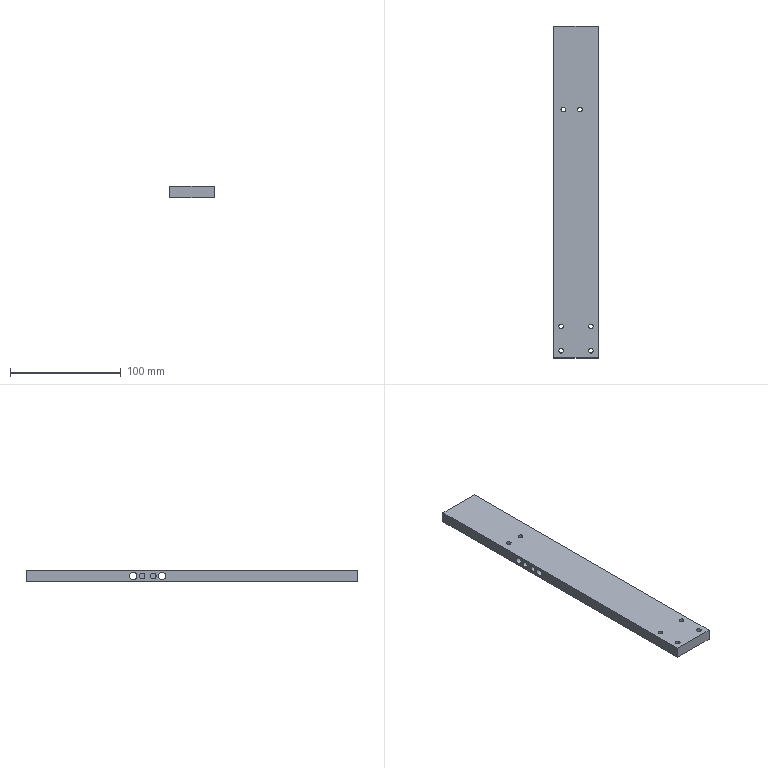Part | STEP file | 11-FG-B04811 | 1 solid | 36 faces | box 40 x 300 x 10 mm | volume 115513 mm3 | cylinder 24 | plane 8 | cone 4 | commonest cylinder face diameters 4.2 x12 5 x8 6.5 x4
STEP:
#1=CARTESIAN_POINT('',(-9.4,224.5,5.));
#2=VERTEX_POINT('',#1);
#3=CARTESIAN_POINT('',(-13.6,224.5,5.));
#4=VERTEX_POINT('',#3);
#5=CARTESIAN_POINT('',(-11.5,224.5,5.));
#6=DIRECTION('',(0.,0.,-1.));
#7=DIRECTION('',(-1.,0.,0.));
#8=AXIS2_PLACEMENT_3D('',#5,#6,#7);
#9=CIRCLE('',#8,2.1);
#10=EDGE_CURVE('',#2,#4,#9,.T.);
#11=ORIENTED_EDGE('',*,*,#10,.F.);
#12=CARTESIAN_POINT('',(-9.4,224.5,-5.));
#13=VERTEX_POINT('',#12);
#14=CARTESIAN_POINT('',(-9.4,224.5,-5.));
#15=DIRECTION('',(0.,0.,-1.));
#16=VECTOR('',#15,1000.);
#17=LINE('',#14,#16);
#18=EDGE_CURVE('',#2,#13,#17,.T.);
#19=ORIENTED_EDGE('',*,*,#18,.T.);
#20=CARTESIAN_POINT('',(-13.6,224.5,-5.));
#21=VERTEX_POINT('',#20);
#22=CARTESIAN_POINT('',(-11.5,224.5,-5.));
#23=DIRECTION('',(0.,0.,-1.));
#24=DIRECTION('',(-1.,0.,0.));
#25=AXIS2_PLACEMENT_3D('',#22,#23,#24);
#26=CIRCLE('',#25,2.1);
#27=EDGE_CURVE('',#13,#21,#26,.T.);
#28=ORIENTED_EDGE('',*,*,#27,.T.);
#29=CARTESIAN_POINT('',(-13.6,224.5,-5.));
#30=DIRECTION('',(0.,0.,-1.));
#31=VECTOR('',#30,1000.);
#32=LINE('',#29,#31);
#33=EDGE_CURVE('',#4,#21,#32,.T.);
#34=ORIENTED_EDGE('',*,*,#33,.F.);
#35=EDGE_LOOP('',(#11,#19,#28,#34));
#36=FACE_OUTER_BOUND('',#35,.T.);
#37=CARTESIAN_POINT('',(-11.5,224.5,-5.));
#38=DIRECTION('',(0.,0.,-1.));
#39=DIRECTION('',(-1.,0.,0.));
#40=AXIS2_PLACEMENT_3D('',#37,#38,#39);
#41=CYLINDRICAL_SURFACE('',#40,2.1);
#42=ADVANCED_FACE('',(#36),#41,.F.);
#43=CARTESIAN_POINT('',(5.6,224.5,5.));
#44=VERTEX_POINT('',#43);
#45=CARTESIAN_POINT('',(1.4,224.5,5.));
#46=VERTEX_POINT('',#45);
#47=CARTESIAN_POINT('',(3.5,224.5,5.));
#48=DIRECTION('',(0.,0.,-1.));
#49=DIRECTION('',(-1.,0.,0.));
#50=AXIS2_PLACEMENT_3D('',#47,#48,#49);
#51=CIRCLE('',#50,2.1);
#52=EDGE_CURVE('',#44,#46,#51,.T.);
#53=ORIENTED_EDGE('',*,*,#52,.F.);
#54=CARTESIAN_POINT('',(5.6,224.5,-5.));
#55=VERTEX_POINT('',#54);
#56=CARTESIAN_POINT('',(5.6,224.5,-5.));
#57=DIRECTION('',(0.,0.,-1.));
#58=VECTOR('',#57,1000.);
#59=LINE('',#56,#58);
#60=EDGE_CURVE('',#44,#55,#59,.T.);
#61=ORIENTED_EDGE('',*,*,#60,.T.);
#62=CARTESIAN_POINT('',(1.4,224.5,-5.));
#63=VERTEX_POINT('',#62);
#64=CARTESIAN_POINT('',(3.5,224.5,-5.));
#65=DIRECTION('',(0.,0.,-1.));
#66=DIRECTION('',(-1.,0.,0.));
#67=AXIS2_PLACEMENT_3D('',#64,#65,#66);
#68=CIRCLE('',#67,2.1);
#69=EDGE_CURVE('',#55,#63,#68,.T.);
#70=ORIENTED_EDGE('',*,*,#69,.T.);
#71=CARTESIAN_POINT('',(1.4,224.5,-5.));
#72=DIRECTION('',(0.,0.,-1.));
#73=VECTOR('',#72,1000.);
#74=LINE('',#71,#73);
#75=EDGE_CURVE('',#46,#63,#74,.T.);
#76=ORIENTED_EDGE('',*,*,#75,.F.);
#77=EDGE_LOOP('',(#53,#61,#70,#76));
#78=FACE_OUTER_BOUND('',#77,.T.);
#79=CARTESIAN_POINT('',(3.5,224.5,-5.));
#80=DIRECTION('',(0.,0.,-1.));
#81=DIRECTION('',(-1.,0.,0.));
#82=AXIS2_PLACEMENT_3D('',#79,#80,#81);
#83=CYLINDRICAL_SURFACE('',#82,2.1);
#84=ADVANCED_FACE('',(#78),#83,.F.);
#85=CARTESIAN_POINT('',(11.4,6.5,-5.));
#86=VERTEX_POINT('',#85);
#87=CARTESIAN_POINT('',(15.6,6.5,-5.));
#88=VERTEX_POINT('',#87);
#89=CARTESIAN_POINT('',(13.5,6.5,-5.));
#90=DIRECTION('',(0.,0.,1.));
#91=DIRECTION('',(1.,0.,0.));
#92=AXIS2_PLACEMENT_3D('',#89,#90,#91);
#93=CIRCLE('',#92,2.1);
#94=EDGE_CURVE('',#86,#88,#93,.T.);
#95=ORIENTED_EDGE('',*,*,#94,.F.);
#96=CARTESIAN_POINT('',(11.4,6.5,5.));
#97=VERTEX_POINT('',#96);
#98=CARTESIAN_POINT('',(11.4,6.5,5.));
#99=DIRECTION('',(0.,0.,1.));
#100=VECTOR('',#99,1000.);
#101=LINE('',#98,#100);
#102=EDGE_CURVE('',#86,#97,#101,.T.);
#103=ORIENTED_EDGE('',*,*,#102,.T.);
#104=CARTESIAN_POINT('',(15.6,6.5,5.));
#105=VERTEX_POINT('',#104);
#106=CARTESIAN_POINT('',(13.5,6.5,5.));
#107=DIRECTION('',(0.,0.,1.));
#108=DIRECTION('',(1.,0.,0.));
#109=AXIS2_PLACEMENT_3D('',#106,#107,#108);
#110=CIRCLE('',#109,2.1);
#111=EDGE_CURVE('',#97,#105,#110,.T.);
#112=ORIENTED_EDGE('',*,*,#111,.T.);
#113=CARTESIAN_POINT('',(15.6,6.5,5.));
#114=DIRECTION('',(0.,0.,1.));
#115=VECTOR('',#114,1000.);
#116=LINE('',#113,#115);
#117=EDGE_CURVE('',#88,#105,#116,.T.);
#118=ORIENTED_EDGE('',*,*,#117,.F.);
#119=EDGE_LOOP('',(#95,#103,#112,#118));
#120=FACE_OUTER_BOUND('',#119,.T.);
#121=CARTESIAN_POINT('',(13.5,6.5,5.));
#122=DIRECTION('',(0.,0.,1.));
#123=DIRECTION('',(1.,0.,0.));
#124=AXIS2_PLACEMENT_3D('',#121,#122,#123);
#125=CYLINDRICAL_SURFACE('',#124,2.1);
#126=ADVANCED_FACE('',(#120),#125,.F.);
#127=CARTESIAN_POINT('',(11.4,28.5,-5.));
#128=VERTEX_POINT('',#127);
#129=CARTESIAN_POINT('',(15.6,28.5,-5.));
#130=VERTEX_POINT('',#129);
#131=CARTESIAN_POINT('',(13.5,28.5,-5.));
#132=DIRECTION('',(0.,0.,1.));
#133=DIRECTION('',(1.,0.,0.));
#134=AXIS2_PLACEMENT_3D('',#131,#132,#133);
#135=CIRCLE('',#134,2.1);
#136=EDGE_CURVE('',#128,#130,#135,.T.);
#137=ORIENTED_EDGE('',*,*,#136,.F.);
#138=CARTESIAN_POINT('',(11.4,28.5,5.));
#139=VERTEX_POINT('',#138);
#140=CARTESIAN_POINT('',(11.4,28.5,5.));
#141=DIRECTION('',(0.,0.,1.));
#142=VECTOR('',#141,1000.);
#143=LINE('',#140,#142);
#144=EDGE_CURVE('',#128,#139,#143,.T.);
#145=ORIENTED_EDGE('',*,*,#144,.T.);
#146=CARTESIAN_POINT('',(15.6,28.5,5.));
#147=VERTEX_POINT('',#146);
#148=CARTESIAN_POINT('',(13.5,28.5,5.));
#149=DIRECTION('',(0.,0.,1.));
#150=DIRECTION('',(1.,0.,0.));
#151=AXIS2_PLACEMENT_3D('',#148,#149,#150);
#152=CIRCLE('',#151,2.1);
#153=EDGE_CURVE('',#139,#147,#152,.T.);
#154=ORIENTED_EDGE('',*,*,#153,.T.);
#155=CARTESIAN_POINT('',(15.6,28.5,5.));
#156=DIRECTION('',(0.,0.,1.));
#157=VECTOR('',#156,1000.);
#158=LINE('',#155,#157);
#159=EDGE_CURVE('',#130,#147,#158,.T.);
#160=ORIENTED_EDGE('',*,*,#159,.F.);
#161=EDGE_LOOP('',(#137,#145,#154,#160));
#162=FACE_OUTER_BOUND('',#161,.T.);
#163=CARTESIAN_POINT('',(13.5,28.5,5.));
#164=DIRECTION('',(0.,0.,1.));
#165=DIRECTION('',(1.,0.,0.));
#166=AXIS2_PLACEMENT_3D('',#163,#164,#165);
#167=CYLINDRICAL_SURFACE('',#166,2.1);
#168=ADVANCED_FACE('',(#162),#167,.F.);
#169=CARTESIAN_POINT('',(-15.6,28.5,-5.));
#170=VERTEX_POINT('',#169);
#171=CARTESIAN_POINT('',(-11.4,28.5,-5.));
#172=VERTEX_POINT('',#171);
#173=CARTESIAN_POINT('',(-13.5,28.5,-5.));
#174=DIRECTION('',(0.,0.,1.));
#175=DIRECTION('',(1.,0.,0.));
#176=AXIS2_PLACEMENT_3D('',#173,#174,#175);
#177=CIRCLE('',#176,2.1);
#178=EDGE_CURVE('',#170,#172,#177,.T.);
#179=ORIENTED_EDGE('',*,*,#178,.F.);
#180=CARTESIAN_POINT('',(-15.6,28.5,5.));
#181=VERTEX_POINT('',#180);
#182=CARTESIAN_POINT('',(-15.6,28.5,5.));
#183=DIRECTION('',(0.,0.,1.));
#184=VECTOR('',#183,1000.);
#185=LINE('',#182,#184);
#186=EDGE_CURVE('',#170,#181,#185,.T.);
#187=ORIENTED_EDGE('',*,*,#186,.T.);
#188=CARTESIAN_POINT('',(-11.4,28.5,5.));
#189=VERTEX_POINT('',#188);
#190=CARTESIAN_POINT('',(-13.5,28.5,5.));
#191=DIRECTION('',(0.,0.,1.));
#192=DIRECTION('',(1.,0.,0.));
#193=AXIS2_PLACEMENT_3D('',#190,#191,#192);
#194=CIRCLE('',#193,2.1);
#195=EDGE_CURVE('',#181,#189,#194,.T.);
#196=ORIENTED_EDGE('',*,*,#195,.T.);
#197=CARTESIAN_POINT('',(-11.4,28.5,5.));
#198=DIRECTION('',(0.,0.,1.));
#199=VECTOR('',#198,1000.);
#200=LINE('',#197,#199);
#201=EDGE_CURVE('',#172,#189,#200,.T.);
#202=ORIENTED_EDGE('',*,*,#201,.F.);
#203=EDGE_LOOP('',(#179,#187,#196,#202));
#204=FACE_OUTER_BOUND('',#203,.T.);
#205=CARTESIAN_POINT('',(-13.5,28.5,5.));
#206=DIRECTION('',(0.,0.,1.));
#207=DIRECTION('',(1.,0.,0.));
#208=AXIS2_PLACEMENT_3D('',#205,#206,#207);
#209=CYLINDRICAL_SURFACE('',#208,2.1);
#210=ADVANCED_FACE('',(#204),#209,.F.);
#211=CARTESIAN_POINT('',(-15.6,6.5,-5.));
#212=VERTEX_POINT('',#211);
#213=CARTESIAN_POINT('',(-11.4,6.5,-5.));
#214=VERTEX_POINT('',#213);
#215=CARTESIAN_POINT('',(-13.5,6.5,-5.));
#216=DIRECTION('',(0.,0.,1.));
#217=DIRECTION('',(1.,0.,0.));
#218=AXIS2_PLACEMENT_3D('',#215,#216,#217);
#219=CIRCLE('',#218,2.1);
#220=EDGE_CURVE('',#212,#214,#219,.T.);
#221=ORIENTED_EDGE('',*,*,#220,.F.);
#222=CARTESIAN_POINT('',(-15.6,6.5,5.));
#223=VERTEX_POINT('',#222);
#224=CARTESIAN_POINT('',(-15.6,6.5,5.));
#225=DIRECTION('',(0.,0.,1.));
#226=VECTOR('',#225,1000.);
#227=LINE('',#224,#226);
#228=EDGE_CURVE('',#212,#223,#227,.T.);
#229=ORIENTED_EDGE('',*,*,#228,.T.);
#230=CARTESIAN_POINT('',(-11.4,6.5,5.));
#231=VERTEX_POINT('',#230);
#232=CARTESIAN_POINT('',(-13.5,6.5,5.));
#233=DIRECTION('',(0.,0.,1.));
#234=DIRECTION('',(1.,0.,0.));
#235=AXIS2_PLACEMENT_3D('',#232,#233,#234);
#236=CIRCLE('',#235,2.1);
#237=EDGE_CURVE('',#223,#231,#236,.T.);
#238=ORIENTED_EDGE('',*,*,#237,.T.);
#239=CARTESIAN_POINT('',(-11.4,6.5,5.));
#240=DIRECTION('',(0.,0.,1.));
#241=VECTOR('',#240,1000.);
#242=LINE('',#239,#241);
#243=EDGE_CURVE('',#214,#231,#242,.T.);
#244=ORIENTED_EDGE('',*,*,#243,.F.);
#245=EDGE_LOOP('',(#221,#229,#238,#244));
#246=FACE_OUTER_BOUND('',#245,.T.);
#247=CARTESIAN_POINT('',(-13.5,6.5,5.));
#248=DIRECTION('',(0.,0.,1.));
#249=DIRECTION('',(1.,0.,0.));
#250=AXIS2_PLACEMENT_3D('',#247,#248,#249);
#251=CYLINDRICAL_SURFACE('',#250,2.1);
#252=ADVANCED_FACE('',(#246),#251,.F.);
#253=CARTESIAN_POINT('',(-12.,285.,-2.5));
#254=VERTEX_POINT('',#253);
#255=CARTESIAN_POINT('',(-12.,285.,2.5));
#256=VERTEX_POINT('',#255);
#257=CARTESIAN_POINT('',(-12.,285.,0.));
#258=DIRECTION('',(0.,1.,0.));
#259=DIRECTION('',(0.,0.,1.));
#260=AXIS2_PLACEMENT_3D('',#257,#258,#259);
#261=CIRCLE('',#260,2.5);
#262=EDGE_CURVE('',#254,#256,#261,.T.);
#263=ORIENTED_EDGE('',*,*,#262,.F.);
#264=CARTESIAN_POINT('',(-12.,300.,-2.5));
#265=VERTEX_POINT('',#264);
#266=CARTESIAN_POINT('',(-12.,300.,-2.5));
#267=DIRECTION('',(0.,1.,0.));
#268=VECTOR('',#267,1000.);
#269=LINE('',#266,#268);
#270=EDGE_CURVE('',#254,#265,#269,.T.);
#271=ORIENTED_EDGE('',*,*,#270,.T.);
#272=CARTESIAN_POINT('',(-12.,300.,2.5));
#273=VERTEX_POINT('',#272);
#274=CARTESIAN_POINT('',(-12.,300.,0.));
#275=DIRECTION('',(0.,1.,0.));
#276=DIRECTION('',(0.,0.,1.));
#277=AXIS2_PLACEMENT_3D('',#274,#275,#276);
#278=CIRCLE('',#277,2.5);
#279=EDGE_CURVE('',#265,#273,#278,.T.);
#280=ORIENTED_EDGE('',*,*,#279,.T.);
#281=CARTESIAN_POINT('',(-12.,300.,2.5));
#282=DIRECTION('',(0.,1.,0.));
#283=VECTOR('',#282,1000.);
#284=LINE('',#281,#283);
#285=EDGE_CURVE('',#256,#273,#284,.T.);
#286=ORIENTED_EDGE('',*,*,#285,.F.);
#287=EDGE_LOOP('',(#263,#271,#280,#286));
#288=FACE_OUTER_BOUND('',#287,.T.);
#289=CARTESIAN_POINT('',(-12.,300.,0.));
#290=DIRECTION('',(0.,1.,0.));
#291=DIRECTION('',(0.,0.,1.));
#292=AXIS2_PLACEMENT_3D('',#289,#290,#291);
#293=CYLINDRICAL_SURFACE('',#292,2.5);
#294=ADVANCED_FACE('',(#288),#293,.F.);
#295=CARTESIAN_POINT('',(-12.,283.498,0.));
#296=VERTEX_POINT('',#295);
#297=CARTESIAN_POINT('',(-12.,285.,2.5));
#298=DIRECTION('',(0.,0.515,0.8572));
#299=VECTOR('',#298,1000.);
#300=LINE('',#297,#299);
#301=EDGE_CURVE('',#296,#256,#300,.T.);
#302=ORIENTED_EDGE('',*,*,#301,.F.);
#303=CARTESIAN_POINT('',(-12.,285.,-2.5));
#304=DIRECTION('',(0.,0.515,-0.8572));
#305=VECTOR('',#304,1000.);
#306=LINE('',#303,#305);
#307=EDGE_CURVE('',#296,#254,#306,.T.);
#308=ORIENTED_EDGE('',*,*,#307,.T.);
#309=ORIENTED_EDGE('',*,*,#262,.T.);
#310=EDGE_LOOP('',(#302,#308,#309));
#311=FACE_OUTER_BOUND('',#310,.T.);
#312=CARTESIAN_POINT('',(-12.,285.,0.));
#313=DIRECTION('',(0.,1.,0.));
#314=DIRECTION('',(0.,0.,1.));
#315=AXIS2_PLACEMENT_3D('',#312,#313,#314);
#316=CONICAL_SURFACE('',#315,2.5,1.03);
#317=ADVANCED_FACE('',(#311),#316,.F.);
#318=CARTESIAN_POINT('',(12.,285.,-2.5));
#319=VERTEX_POINT('',#318);
#320=CARTESIAN_POINT('',(12.,285.,2.5));
#321=VERTEX_POINT('',#320);
#322=CARTESIAN_POINT('',(12.,285.,0.));
#323=DIRECTION('',(0.,1.,0.));
#324=DIRECTION('',(0.,0.,1.));
#325=AXIS2_PLACEMENT_3D('',#322,#323,#324);
#326=CIRCLE('',#325,2.5);
#327=EDGE_CURVE('',#319,#321,#326,.T.);
#328=ORIENTED_EDGE('',*,*,#327,.F.);
#329=CARTESIAN_POINT('',(12.,300.,-2.5));
#330=VERTEX_POINT('',#329);
#331=CARTESIAN_POINT('',(12.,300.,-2.5));
#332=DIRECTION('',(0.,1.,0.));
#333=VECTOR('',#332,1000.);
#334=LINE('',#331,#333);
#335=EDGE_CURVE('',#319,#330,#334,.T.);
#336=ORIENTED_EDGE('',*,*,#335,.T.);
#337=CARTESIAN_POINT('',(12.,300.,2.5));
#338=VERTEX_POINT('',#337);
#339=CARTESIAN_POINT('',(12.,300.,0.));
#340=DIRECTION('',(0.,1.,0.));
#341=DIRECTION('',(0.,0.,1.));
#342=AXIS2_PLACEMENT_3D('',#339,#340,#341);
#343=CIRCLE('',#342,2.5);
#344=EDGE_CURVE('',#330,#338,#343,.T.);
#345=ORIENTED_EDGE('',*,*,#344,.T.);
#346=CARTESIAN_POINT('',(12.,300.,2.5));
#347=DIRECTION('',(0.,1.,0.));
#348=VECTOR('',#347,1000.);
#349=LINE('',#346,#348);
#350=EDGE_CURVE('',#321,#338,#349,.T.);
#351=ORIENTED_EDGE('',*,*,#350,.F.);
#352=EDGE_LOOP('',(#328,#336,#345,#351));
#353=FACE_OUTER_BOUND('',#352,.T.);
#354=CARTESIAN_POINT('',(12.,300.,0.));
#355=DIRECTION('',(0.,1.,0.));
#356=DIRECTION('',(0.,0.,1.));
#357=AXIS2_PLACEMENT_3D('',#354,#355,#356);
#358=CYLINDRICAL_SURFACE('',#357,2.5);
#359=ADVANCED_FACE('',(#353),#358,.F.);
#360=CARTESIAN_POINT('',(12.,283.498,0.));
#361=VERTEX_POINT('',#360);
#362=CARTESIAN_POINT('',(12.,285.,2.5));
#363=DIRECTION('',(0.,0.515,0.8572));
#364=VECTOR('',#363,1000.);
#365=LINE('',#362,#364);
#366=EDGE_CURVE('',#361,#321,#365,.T.);
#367=ORIENTED_EDGE('',*,*,#366,.F.);
#368=CARTESIAN_POINT('',(12.,285.,-2.5));
#369=DIRECTION('',(0.,0.515,-0.8572));
#370=VECTOR('',#369,1000.);
#371=LINE('',#368,#370);
#372=EDGE_CURVE('',#361,#319,#371,.T.);
#373=ORIENTED_EDGE('',*,*,#372,.T.);
#374=ORIENTED_EDGE('',*,*,#327,.T.);
#375=EDGE_LOOP('',(#367,#373,#374));
#376=FACE_OUTER_BOUND('',#375,.T.);
#377=CARTESIAN_POINT('',(12.,285.,0.));
#378=DIRECTION('',(0.,1.,0.));
#379=DIRECTION('',(0.,0.,1.));
#380=AXIS2_PLACEMENT_3D('',#377,#378,#379);
#381=CONICAL_SURFACE('',#380,2.5,1.03);
#382=ADVANCED_FACE('',(#376),#381,.F.);
#383=CARTESIAN_POINT('',(-10.,195.,-2.5));
#384=VERTEX_POINT('',#383);
#385=CARTESIAN_POINT('',(-10.,195.,2.5));
#386=VERTEX_POINT('',#385);
#387=CARTESIAN_POINT('',(-10.,195.,0.));
#388=DIRECTION('',(-1.,0.,0.));
#389=DIRECTION('',(0.,0.,1.));
#390=AXIS2_PLACEMENT_3D('',#387,#388,#389);
#391=CIRCLE('',#390,2.5);
#392=EDGE_CURVE('',#384,#386,#391,.T.);
#393=ORIENTED_EDGE('',*,*,#392,.F.);
#394=CARTESIAN_POINT('',(-20.,195.,-2.5));
#395=VERTEX_POINT('',#394);
#396=CARTESIAN_POINT('',(-10.,195.,-2.5));
#397=DIRECTION('',(-1.,0.,0.));
#398=VECTOR('',#397,1000.);
#399=LINE('',#396,#398);
#400=EDGE_CURVE('',#384,#395,#399,.T.);
#401=ORIENTED_EDGE('',*,*,#400,.T.);
#402=CARTESIAN_POINT('',(-20.,195.,2.5));
#403=VERTEX_POINT('',#402);
#404=CARTESIAN_POINT('',(-20.,195.,0.));
#405=DIRECTION('',(-1.,0.,0.));
#406=DIRECTION('',(0.,0.,1.));
#407=AXIS2_PLACEMENT_3D('',#404,#405,#406);
#408=CIRCLE('',#407,2.5);
#409=EDGE_CURVE('',#395,#403,#408,.T.);
#410=ORIENTED_EDGE('',*,*,#409,.T.);
#411=CARTESIAN_POINT('',(-10.,195.,2.5));
#412=DIRECTION('',(-1.,0.,0.));
#413=VECTOR('',#412,1000.);
#414=LINE('',#411,#413);
#415=EDGE_CURVE('',#386,#403,#414,.T.);
#416=ORIENTED_EDGE('',*,*,#415,.F.);
#417=EDGE_LOOP('',(#393,#401,#410,#416));
#418=FACE_OUTER_BOUND('',#417,.T.);
#419=CARTESIAN_POINT('',(-10.,195.,0.));
#420=DIRECTION('',(-1.,0.,0.));
#421=DIRECTION('',(0.,0.,1.));
#422=AXIS2_PLACEMENT_3D('',#419,#420,#421);
#423=CYLINDRICAL_SURFACE('',#422,2.5);
#424=ADVANCED_FACE('',(#418),#423,.F.);
#425=CARTESIAN_POINT('',(-10.,185.,-2.5));
#426=VERTEX_POINT('',#425);
#427=CARTESIAN_POINT('',(-10.,185.,2.5));
#428=VERTEX_POINT('',#427);
#429=CARTESIAN_POINT('',(-10.,185.,0.));
#430=DIRECTION('',(-1.,0.,0.));
#431=DIRECTION('',(0.,0.,1.));
#432=AXIS2_PLACEMENT_3D('',#429,#430,#431);
#433=CIRCLE('',#432,2.5);
#434=EDGE_CURVE('',#426,#428,#433,.T.);
#435=ORIENTED_EDGE('',*,*,#434,.F.);
#436=CARTESIAN_POINT('',(-20.,185.,-2.5));
#437=VERTEX_POINT('',#436);
#438=CARTESIAN_POINT('',(-10.,185.,-2.5));
#439=DIRECTION('',(-1.,0.,0.));
#440=VECTOR('',#439,1000.);
#441=LINE('',#438,#440);
#442=EDGE_CURVE('',#426,#437,#441,.T.);
#443=ORIENTED_EDGE('',*,*,#442,.T.);
#444=CARTESIAN_POINT('',(-20.,185.,2.5));
#445=VERTEX_POINT('',#444);
#446=CARTESIAN_POINT('',(-20.,185.,0.));
#447=DIRECTION('',(-1.,0.,0.));
#448=DIRECTION('',(0.,0.,1.));
#449=AXIS2_PLACEMENT_3D('',#446,#447,#448);
#450=CIRCLE('',#449,2.5);
#451=EDGE_CURVE('',#437,#445,#450,.T.);
#452=ORIENTED_EDGE('',*,*,#451,.T.);
#453=CARTESIAN_POINT('',(-10.,185.,2.5));
#454=DIRECTION('',(-1.,0.,0.));
#455=VECTOR('',#454,1000.);
#456=LINE('',#453,#455);
#457=EDGE_CURVE('',#428,#445,#456,.T.);
#458=ORIENTED_EDGE('',*,*,#457,.F.);
#459=EDGE_LOOP('',(#435,#443,#452,#458));
#460=FACE_OUTER_BOUND('',#459,.T.);
#461=CARTESIAN_POINT('',(-10.,185.,0.));
#462=DIRECTION('',(-1.,0.,0.));
#463=DIRECTION('',(0.,0.,1.));
#464=AXIS2_PLACEMENT_3D('',#461,#462,#463);
#465=CYLINDRICAL_SURFACE('',#464,2.5);
#466=ADVANCED_FACE('',(#460),#465,.F.);
#467=CARTESIAN_POINT('',(-20.,177.,3.25));
#468=VERTEX_POINT('',#467);
#469=CARTESIAN_POINT('',(-20.,177.,-3.25));
#470=VERTEX_POINT('',#469);
#471=CARTESIAN_POINT('',(-20.,177.,0.));
#472=DIRECTION('',(1.,0.,0.));
#473=DIRECTION('',(0.,0.,-1.));
#474=AXIS2_PLACEMENT_3D('',#471,#472,#473);
#475=CIRCLE('',#474,3.25);
#476=EDGE_CURVE('',#468,#470,#475,.T.);
#477=ORIENTED_EDGE('',*,*,#476,.F.);
#478=CARTESIAN_POINT('',(20.,177.,3.25));
#479=VERTEX_POINT('',#478);
#480=CARTESIAN_POINT('',(-85.,177.,3.25));
#481=DIRECTION('',(1.,0.,0.));
#482=VECTOR('',#481,1000.);
#483=LINE('',#480,#482);
#484=EDGE_CURVE('',#468,#479,#483,.T.);
#485=ORIENTED_EDGE('',*,*,#484,.T.);
#486=CARTESIAN_POINT('',(20.,177.,-3.25));
#487=VERTEX_POINT('',#486);
#488=CARTESIAN_POINT('',(20.,177.,0.));
#489=DIRECTION('',(1.,0.,0.));
#490=DIRECTION('',(0.,0.,-1.));
#491=AXIS2_PLACEMENT_3D('',#488,#489,#490);
#492=CIRCLE('',#491,3.25);
#493=EDGE_CURVE('',#479,#487,#492,.T.);
#494=ORIENTED_EDGE('',*,*,#493,.T.);
#495=CARTESIAN_POINT('',(-85.,177.,-3.25));
#496=DIRECTION('',(1.,0.,0.));
#497=VECTOR('',#496,1000.);
#498=LINE('',#495,#497);
#499=EDGE_CURVE('',#470,#487,#498,.T.);
#500=ORIENTED_EDGE('',*,*,#499,.F.);
#501=EDGE_LOOP('',(#477,#485,#494,#500));
#502=FACE_OUTER_BOUND('',#501,.T.);
#503=CARTESIAN_POINT('',(-85.,177.,0.));
#504=DIRECTION('',(1.,0.,0.));
#505=DIRECTION('',(0.,0.,-1.));
#506=AXIS2_PLACEMENT_3D('',#503,#504,#505);
#507=CYLINDRICAL_SURFACE('',#506,3.25);
#508=ADVANCED_FACE('',(#502),#507,.F.);
#509=CARTESIAN_POINT('',(-20.,203.,3.25));
#510=VERTEX_POINT('',#509);
#511=CARTESIAN_POINT('',(-20.,203.,-3.25));
#512=VERTEX_POINT('',#511);
#513=CARTESIAN_POINT('',(-20.,203.,0.));
#514=DIRECTION('',(1.,0.,0.));
#515=DIRECTION('',(0.,0.,-1.));
#516=AXIS2_PLACEMENT_3D('',#513,#514,#515);
#517=CIRCLE('',#516,3.25);
#518=EDGE_CURVE('',#510,#512,#517,.T.);
#519=ORIENTED_EDGE('',*,*,#518,.F.);
#520=CARTESIAN_POINT('',(20.,203.,3.25));
#521=VERTEX_POINT('',#520);
#522=CARTESIAN_POINT('',(-85.,203.,3.25));
#523=DIRECTION('',(1.,0.,0.));
#524=VECTOR('',#523,1000.);
#525=LINE('',#522,#524);
#526=EDGE_CURVE('',#510,#521,#525,.T.);
#527=ORIENTED_EDGE('',*,*,#526,.T.);
#528=CARTESIAN_POINT('',(20.,203.,-3.25));
#529=VERTEX_POINT('',#528);
#530=CARTESIAN_POINT('',(20.,203.,0.));
#531=DIRECTION('',(1.,0.,0.));
#532=DIRECTION('',(0.,0.,-1.));
#533=AXIS2_PLACEMENT_3D('',#530,#531,#532);
#534=CIRCLE('',#533,3.25);
#535=EDGE_CURVE('',#521,#529,#534,.T.);
#536=ORIENTED_EDGE('',*,*,#535,.T.);
#537=CARTESIAN_POINT('',(-85.,203.,-3.25));
#538=DIRECTION('',(1.,0.,0.));
#539=VECTOR('',#538,1000.);
#540=LINE('',#537,#539);
#541=EDGE_CURVE('',#512,#529,#540,.T.);
#542=ORIENTED_EDGE('',*,*,#541,.F.);
#543=EDGE_LOOP('',(#519,#527,#536,#542));
#544=FACE_OUTER_BOUND('',#543,.T.);
#545=CARTESIAN_POINT('',(-85.,203.,0.));
#546=DIRECTION('',(1.,0.,0.));
#547=DIRECTION('',(0.,0.,-1.));
#548=AXIS2_PLACEMENT_3D('',#545,#546,#547);
#549=CYLINDRICAL_SURFACE('',#548,3.25);
#550=ADVANCED_FACE('',(#544),#549,.F.);
#551=CARTESIAN_POINT('',(20.,177.,0.));
#552=DIRECTION('',(1.,0.,0.));
#553=DIRECTION('',(0.,0.,-1.));
#554=AXIS2_PLACEMENT_3D('',#551,#552,#553);
#555=CIRCLE('',#554,3.25);
#556=EDGE_CURVE('',#487,#479,#555,.T.);
#557=ORIENTED_EDGE('',*,*,#556,.F.);
#558=ORIENTED_EDGE('',*,*,#493,.F.);
#559=EDGE_LOOP('',(#557,#558));
#560=FACE_BOUND('',#559,.T.);
#561=CARTESIAN_POINT('',(20.,203.,0.));
#562=DIRECTION('',(1.,0.,0.));
#563=DIRECTION('',(0.,0.,-1.));
#564=AXIS2_PLACEMENT_3D('',#561,#562,#563);
#565=CIRCLE('',#564,3.25);
#566=EDGE_CURVE('',#529,#521,#565,.T.);
#567=ORIENTED_EDGE('',*,*,#566,.F.);
#568=ORIENTED_EDGE('',*,*,#535,.F.);
#569=EDGE_LOOP('',(#567,#568));
#570=FACE_BOUND('',#569,.T.);
#571=CARTESIAN_POINT('',(20.,0.,5.));
#572=VERTEX_POINT('',#571);
#573=CARTESIAN_POINT('',(20.,0.,-5.));
#574=VERTEX_POINT('',#573);
#575=CARTESIAN_POINT('',(20.,0.,-5.));
#576=DIRECTION('',(0.,0.,-1.));
#577=VECTOR('',#576,1000.);
#578=LINE('',#575,#577);
#579=EDGE_CURVE('',#572,#574,#578,.T.);
#580=ORIENTED_EDGE('',*,*,#579,.T.);
#581=CARTESIAN_POINT('',(20.,300.,-5.));
#582=VERTEX_POINT('',#581);
#583=CARTESIAN_POINT('',(20.,300.,-5.));
#584=DIRECTION('',(0.,-1.,0.));
#585=VECTOR('',#584,1000.);
#586=LINE('',#583,#585);
#587=EDGE_CURVE('',#582,#574,#586,.T.);
#588=ORIENTED_EDGE('',*,*,#587,.F.);
#589=CARTESIAN_POINT('',(20.,300.,5.));
#590=VERTEX_POINT('',#589);
#591=CARTESIAN_POINT('',(20.,300.,-5.));
#592=DIRECTION('',(0.,0.,-1.));
#593=VECTOR('',#592,1000.);
#594=LINE('',#591,#593);
#595=EDGE_CURVE('',#590,#582,#594,.T.);
#596=ORIENTED_EDGE('',*,*,#595,.F.);
#597=CARTESIAN_POINT('',(20.,300.,5.));
#598=DIRECTION('',(0.,-1.,0.));
#599=VECTOR('',#598,1000.);
#600=LINE('',#597,#599);
#601=EDGE_CURVE('',#590,#572,#600,.T.);
#602=ORIENTED_EDGE('',*,*,#601,.T.);
#603=EDGE_LOOP('',(#580,#588,#596,#602));
#604=FACE_OUTER_BOUND('',#603,.T.);
#605=CARTESIAN_POINT('',(20.,300.,-5.));
#606=DIRECTION('',(-1.,0.,0.));
#607=DIRECTION('',(0.,0.,1.));
#608=AXIS2_PLACEMENT_3D('',#605,#606,#607);
#609=PLANE('',#608);
#610=ADVANCED_FACE('',(#560,#570,#604),#609,.F.);
#611=CARTESIAN_POINT('',(-11.5,224.5,-5.));
#612=DIRECTION('',(0.,0.,-1.));
#613=DIRECTION('',(-1.,0.,0.));
#614=AXIS2_PLACEMENT_3D('',#611,#612,#613);
#615=CIRCLE('',#614,2.1);
#616=EDGE_CURVE('',#21,#13,#615,.T.);
#617=ORIENTED_EDGE('',*,*,#616,.F.);
#618=ORIENTED_EDGE('',*,*,#27,.F.);
#619=EDGE_LOOP('',(#617,#618));
#620=FACE_BOUND('',#619,.T.);
#621=CARTESIAN_POINT('',(3.5,224.5,-5.));
#622=DIRECTION('',(0.,0.,-1.));
#623=DIRECTION('',(-1.,0.,0.));
#624=AXIS2_PLACEMENT_3D('',#621,#622,#623);
#625=CIRCLE('',#624,2.1);
#626=EDGE_CURVE('',#63,#55,#625,.T.);
#627=ORIENTED_EDGE('',*,*,#626,.F.);
#628=ORIENTED_EDGE('',*,*,#69,.F.);
#629=EDGE_LOOP('',(#627,#628));
#630=FACE_BOUND('',#629,.T.);
#631=CARTESIAN_POINT('',(13.5,6.5,-5.));
#632=DIRECTION('',(0.,0.,1.));
#633=DIRECTION('',(1.,0.,0.));
#634=AXIS2_PLACEMENT_3D('',#631,#632,#633);
#635=CIRCLE('',#634,2.1);
#636=EDGE_CURVE('',#88,#86,#635,.T.);
#637=ORIENTED_EDGE('',*,*,#636,.T.);
#638=ORIENTED_EDGE('',*,*,#94,.T.);
#639=EDGE_LOOP('',(#637,#638));
#640=FACE_BOUND('',#639,.T.);
#641=CARTESIAN_POINT('',(13.5,28.5,-5.));
#642=DIRECTION('',(0.,0.,1.));
#643=DIRECTION('',(1.,0.,0.));
#644=AXIS2_PLACEMENT_3D('',#641,#642,#643);
#645=CIRCLE('',#644,2.1);
#646=EDGE_CURVE('',#130,#128,#645,.T.);
#647=ORIENTED_EDGE('',*,*,#646,.T.);
#648=ORIENTED_EDGE('',*,*,#136,.T.);
#649=EDGE_LOOP('',(#647,#648));
#650=FACE_BOUND('',#649,.T.);
#651=CARTESIAN_POINT('',(-13.5,28.5,-5.));
#652=DIRECTION('',(0.,0.,1.));
#653=DIRECTION('',(1.,0.,0.));
#654=AXIS2_PLACEMENT_3D('',#651,#652,#653);
#655=CIRCLE('',#654,2.1);
#656=EDGE_CURVE('',#172,#170,#655,.T.);
#657=ORIENTED_EDGE('',*,*,#656,.T.);
#658=ORIENTED_EDGE('',*,*,#178,.T.);
#659=EDGE_LOOP('',(#657,#658));
#660=FACE_BOUND('',#659,.T.);
#661=CARTESIAN_POINT('',(-13.5,6.5,-5.));
#662=DIRECTION('',(0.,0.,1.));
#663=DIRECTION('',(1.,0.,0.));
#664=AXIS2_PLACEMENT_3D('',#661,#662,#663);
#665=CIRCLE('',#664,2.1);
#666=EDGE_CURVE('',#214,#212,#665,.T.);
#667=ORIENTED_EDGE('',*,*,#666,.T.);
#668=ORIENTED_EDGE('',*,*,#220,.T.);
#669=EDGE_LOOP('',(#667,#668));
#670=FACE_BOUND('',#669,.T.);
#671=CARTESIAN_POINT('',(-20.,0.,-5.));
#672=VERTEX_POINT('',#671);
#673=CARTESIAN_POINT('',(-20.,0.,-5.));
#674=DIRECTION('',(-1.,0.,0.));
#675=VECTOR('',#674,1000.);
#676=LINE('',#673,#675);
#677=EDGE_CURVE('',#574,#672,#676,.T.);
#678=ORIENTED_EDGE('',*,*,#677,.T.);
#679=CARTESIAN_POINT('',(-20.,300.,-5.));
#680=VERTEX_POINT('',#679);
#681=CARTESIAN_POINT('',(-20.,300.,-5.));
#682=DIRECTION('',(0.,-1.,0.));
#683=VECTOR('',#682,1000.);
#684=LINE('',#681,#683);
#685=EDGE_CURVE('',#680,#672,#684,.T.);
#686=ORIENTED_EDGE('',*,*,#685,.F.);
#687=CARTESIAN_POINT('',(-20.,300.,-5.));
#688=DIRECTION('',(-1.,0.,0.));
#689=VECTOR('',#688,1000.);
#690=LINE('',#687,#689);
#691=EDGE_CURVE('',#582,#680,#690,.T.);
#692=ORIENTED_EDGE('',*,*,#691,.F.);
#693=ORIENTED_EDGE('',*,*,#587,.T.);
#694=EDGE_LOOP('',(#678,#686,#692,#693));
#695=FACE_OUTER_BOUND('',#694,.T.);
#696=CARTESIAN_POINT('',(-20.,300.,-5.));
#697=DIRECTION('',(0.,0.,1.));
#698=DIRECTION('',(1.,0.,0.));
#699=AXIS2_PLACEMENT_3D('',#696,#697,#698);
#700=PLANE('',#699);
#701=ADVANCED_FACE('',(#620,#630,#640,#650,#660,#670,#695),#700,.F.);
#702=CARTESIAN_POINT('',(-20.,195.,0.));
#703=DIRECTION('',(-1.,0.,0.));
#704=DIRECTION('',(0.,0.,1.));
#705=AXIS2_PLACEMENT_3D('',#702,#703,#704);
#706=CIRCLE('',#705,2.5);
#707=EDGE_CURVE('',#403,#395,#706,.T.);
#708=ORIENTED_EDGE('',*,*,#707,.F.);
#709=ORIENTED_EDGE('',*,*,#409,.F.);
#710=EDGE_LOOP('',(#708,#709));
#711=FACE_BOUND('',#710,.T.);
#712=CARTESIAN_POINT('',(-20.,185.,0.));
#713=DIRECTION('',(-1.,0.,0.));
#714=DIRECTION('',(0.,0.,1.));
#715=AXIS2_PLACEMENT_3D('',#712,#713,#714);
#716=CIRCLE('',#715,2.5);
#717=EDGE_CURVE('',#445,#437,#716,.T.);
#718=ORIENTED_EDGE('',*,*,#717,.F.);
#719=ORIENTED_EDGE('',*,*,#451,.F.);
#720=EDGE_LOOP('',(#718,#719));
#721=FACE_BOUND('',#720,.T.);
#722=CARTESIAN_POINT('',(-20.,177.,0.));
#723=DIRECTION('',(1.,0.,0.));
#724=DIRECTION('',(0.,0.,-1.));
#725=AXIS2_PLACEMENT_3D('',#722,#723,#724);
#726=CIRCLE('',#725,3.25);
#727=EDGE_CURVE('',#470,#468,#726,.T.);
#728=ORIENTED_EDGE('',*,*,#727,.T.);
#729=ORIENTED_EDGE('',*,*,#476,.T.);
#730=EDGE_LOOP('',(#728,#729));
#731=FACE_BOUND('',#730,.T.);
#732=CARTESIAN_POINT('',(-20.,203.,0.));
#733=DIRECTION('',(1.,0.,0.));
#734=DIRECTION('',(0.,0.,-1.));
#735=AXIS2_PLACEMENT_3D('',#732,#733,#734);
#736=CIRCLE('',#735,3.25);
#737=EDGE_CURVE('',#512,#510,#736,.T.);
#738=ORIENTED_EDGE('',*,*,#737,.T.);
#739=ORIENTED_EDGE('',*,*,#518,.T.);
#740=EDGE_LOOP('',(#738,#739));
#741=FACE_BOUND('',#740,.T.);
#742=CARTESIAN_POINT('',(-20.,0.,5.));
#743=VERTEX_POINT('',#742);
#744=CARTESIAN_POINT('',(-20.,0.,-5.));
#745=DIRECTION('',(0.,0.,1.));
#746=VECTOR('',#745,1000.);
#747=LINE('',#744,#746);
#748=EDGE_CURVE('',#672,#743,#747,.T.);
#749=ORIENTED_EDGE('',*,*,#748,.T.);
#750=CARTESIAN_POINT('',(-20.,300.,5.));
#751=VERTEX_POINT('',#750);
#752=CARTESIAN_POINT('',(-20.,300.,5.));
#753=DIRECTION('',(0.,-1.,0.));
#754=VECTOR('',#753,1000.);
#755=LINE('',#752,#754);
#756=EDGE_CURVE('',#751,#743,#755,.T.);
#757=ORIENTED_EDGE('',*,*,#756,.F.);
#758=CARTESIAN_POINT('',(-20.,300.,-5.));
#759=DIRECTION('',(0.,0.,1.));
#760=VECTOR('',#759,1000.);
#761=LINE('',#758,#760);
#762=EDGE_CURVE('',#680,#751,#761,.T.);
#763=ORIENTED_EDGE('',*,*,#762,.F.);
#764=ORIENTED_EDGE('',*,*,#685,.T.);
#765=EDGE_LOOP('',(#749,#757,#763,#764));
#766=FACE_OUTER_BOUND('',#765,.T.);
#767=CARTESIAN_POINT('',(-20.,300.,-5.));
#768=DIRECTION('',(1.,0.,0.));
#769=DIRECTION('',(0.,0.,-1.));
#770=AXIS2_PLACEMENT_3D('',#767,#768,#769);
#771=PLANE('',#770);
#772=ADVANCED_FACE('',(#711,#721,#731,#741,#766),#771,.F.);
#773=CARTESIAN_POINT('',(-11.5,224.5,5.));
#774=DIRECTION('',(0.,0.,-1.));
#775=DIRECTION('',(-1.,0.,0.));
#776=AXIS2_PLACEMENT_3D('',#773,#774,#775);
#777=CIRCLE('',#776,2.1);
#778=EDGE_CURVE('',#4,#2,#777,.T.);
#779=ORIENTED_EDGE('',*,*,#778,.T.);
#780=ORIENTED_EDGE('',*,*,#10,.T.);
#781=EDGE_LOOP('',(#779,#780));
#782=FACE_BOUND('',#781,.T.);
#783=CARTESIAN_POINT('',(3.5,224.5,5.));
#784=DIRECTION('',(0.,0.,-1.));
#785=DIRECTION('',(-1.,0.,0.));
#786=AXIS2_PLACEMENT_3D('',#783,#784,#785);
#787=CIRCLE('',#786,2.1);
#788=EDGE_CURVE('',#46,#44,#787,.T.);
#789=ORIENTED_EDGE('',*,*,#788,.T.);
#790=ORIENTED_EDGE('',*,*,#52,.T.);
#791=EDGE_LOOP('',(#789,#790));
#792=FACE_BOUND('',#791,.T.);
#793=CARTESIAN_POINT('',(13.5,6.5,5.));
#794=DIRECTION('',(0.,0.,1.));
#795=DIRECTION('',(1.,0.,0.));
#796=AXIS2_PLACEMENT_3D('',#793,#794,#795);
#797=CIRCLE('',#796,2.1);
#798=EDGE_CURVE('',#105,#97,#797,.T.);
#799=ORIENTED_EDGE('',*,*,#798,.F.);
#800=ORIENTED_EDGE('',*,*,#111,.F.);
#801=EDGE_LOOP('',(#799,#800));
#802=FACE_BOUND('',#801,.T.);
#803=CARTESIAN_POINT('',(13.5,28.5,5.));
#804=DIRECTION('',(0.,0.,1.));
#805=DIRECTION('',(1.,0.,0.));
#806=AXIS2_PLACEMENT_3D('',#803,#804,#805);
#807=CIRCLE('',#806,2.1);
#808=EDGE_CURVE('',#147,#139,#807,.T.);
#809=ORIENTED_EDGE('',*,*,#808,.F.);
#810=ORIENTED_EDGE('',*,*,#153,.F.);
#811=EDGE_LOOP('',(#809,#810));
#812=FACE_BOUND('',#811,.T.);
#813=CARTESIAN_POINT('',(-13.5,28.5,5.));
#814=DIRECTION('',(0.,0.,1.));
#815=DIRECTION('',(1.,0.,0.));
#816=AXIS2_PLACEMENT_3D('',#813,#814,#815);
#817=CIRCLE('',#816,2.1);
#818=EDGE_CURVE('',#189,#181,#817,.T.);
#819=ORIENTED_EDGE('',*,*,#818,.F.);
#820=ORIENTED_EDGE('',*,*,#195,.F.);
#821=EDGE_LOOP('',(#819,#820));
#822=FACE_BOUND('',#821,.T.);
#823=CARTESIAN_POINT('',(-13.5,6.5,5.));
#824=DIRECTION('',(0.,0.,1.));
#825=DIRECTION('',(1.,0.,0.));
#826=AXIS2_PLACEMENT_3D('',#823,#824,#825);
#827=CIRCLE('',#826,2.1);
#828=EDGE_CURVE('',#231,#223,#827,.T.);
#829=ORIENTED_EDGE('',*,*,#828,.F.);
#830=ORIENTED_EDGE('',*,*,#237,.F.);
#831=EDGE_LOOP('',(#829,#830));
#832=FACE_BOUND('',#831,.T.);
#833=CARTESIAN_POINT('',(-20.,0.,5.));
#834=DIRECTION('',(1.,0.,0.));
#835=VECTOR('',#834,1000.);
#836=LINE('',#833,#835);
#837=EDGE_CURVE('',#743,#572,#836,.T.);
#838=ORIENTED_EDGE('',*,*,#837,.T.);
#839=ORIENTED_EDGE('',*,*,#601,.F.);
#840=CARTESIAN_POINT('',(-20.,300.,5.));
#841=DIRECTION('',(1.,0.,0.));
#842=VECTOR('',#841,1000.);
#843=LINE('',#840,#842);
#844=EDGE_CURVE('',#751,#590,#843,.T.);
#845=ORIENTED_EDGE('',*,*,#844,.F.);
#846=ORIENTED_EDGE('',*,*,#756,.T.);
#847=EDGE_LOOP('',(#838,#839,#845,#846));
#848=FACE_OUTER_BOUND('',#847,.T.);
#849=CARTESIAN_POINT('',(-20.,300.,5.));
#850=DIRECTION('',(0.,0.,-1.));
#851=DIRECTION('',(-1.,0.,0.));
#852=AXIS2_PLACEMENT_3D('',#849,#850,#851);
#853=PLANE('',#852);
#854=ADVANCED_FACE('',(#782,#792,#802,#812,#822,#832,#848),#853,.F.);
#855=CARTESIAN_POINT('',(-12.,300.,0.));
#856=DIRECTION('',(0.,1.,0.));
#857=DIRECTION('',(0.,0.,1.));
#858=AXIS2_PLACEMENT_3D('',#855,#856,#857);
#859=CIRCLE('',#858,2.5);
#860=EDGE_CURVE('',#273,#265,#859,.T.);
#861=ORIENTED_EDGE('',*,*,#860,.F.);
#862=ORIENTED_EDGE('',*,*,#279,.F.);
#863=EDGE_LOOP('',(#861,#862));
#864=FACE_BOUND('',#863,.T.);
#865=CARTESIAN_POINT('',(12.,300.,0.));
#866=DIRECTION('',(0.,1.,0.));
#867=DIRECTION('',(0.,0.,1.));
#868=AXIS2_PLACEMENT_3D('',#865,#866,#867);
#869=CIRCLE('',#868,2.5);
#870=EDGE_CURVE('',#338,#330,#869,.T.);
#871=ORIENTED_EDGE('',*,*,#870,.F.);
#872=ORIENTED_EDGE('',*,*,#344,.F.);
#873=EDGE_LOOP('',(#871,#872));
#874=FACE_BOUND('',#873,.T.);
#875=ORIENTED_EDGE('',*,*,#595,.T.);
#876=ORIENTED_EDGE('',*,*,#691,.T.);
#877=ORIENTED_EDGE('',*,*,#762,.T.);
#878=ORIENTED_EDGE('',*,*,#844,.T.);
#879=EDGE_LOOP('',(#875,#876,#877,#878));
#880=FACE_OUTER_BOUND('',#879,.T.);
#881=CARTESIAN_POINT('',(0.,300.,0.));
#882=DIRECTION('',(0.,1.,0.));
#883=DIRECTION('',(0.,0.,1.));
#884=AXIS2_PLACEMENT_3D('',#881,#882,#883);
#885=PLANE('',#884);
#886=ADVANCED_FACE('',(#864,#874,#880),#885,.T.);
#887=ORIENTED_EDGE('',*,*,#579,.F.);
#888=ORIENTED_EDGE('',*,*,#837,.F.);
#889=ORIENTED_EDGE('',*,*,#748,.F.);
#890=ORIENTED_EDGE('',*,*,#677,.F.);
#891=EDGE_LOOP('',(#887,#888,#889,#890));
#892=FACE_OUTER_BOUND('',#891,.T.);
#893=CARTESIAN_POINT('',(0.,0.,0.));
#894=DIRECTION('',(0.,1.,0.));
#895=DIRECTION('',(0.,0.,1.));
#896=AXIS2_PLACEMENT_3D('',#893,#894,#895);
#897=PLANE('',#896);
#898=ADVANCED_FACE('',(#892),#897,.F.);
#899=ORIENTED_EDGE('',*,*,#526,.F.);
#900=ORIENTED_EDGE('',*,*,#737,.F.);
#901=ORIENTED_EDGE('',*,*,#541,.T.);
#902=ORIENTED_EDGE('',*,*,#566,.T.);
#903=EDGE_LOOP('',(#899,#900,#901,#902));
#904=FACE_OUTER_BOUND('',#903,.T.);
#905=CARTESIAN_POINT('',(-85.,203.,0.));
#906=DIRECTION('',(1.,0.,0.));
#907=DIRECTION('',(0.,0.,-1.));
#908=AXIS2_PLACEMENT_3D('',#905,#906,#907);
#909=CYLINDRICAL_SURFACE('',#908,3.25);
#910=ADVANCED_FACE('',(#904),#909,.F.);
#911=ORIENTED_EDGE('',*,*,#484,.F.);
#912=ORIENTED_EDGE('',*,*,#727,.F.);
#913=ORIENTED_EDGE('',*,*,#499,.T.);
#914=ORIENTED_EDGE('',*,*,#556,.T.);
#915=EDGE_LOOP('',(#911,#912,#913,#914));
#916=FACE_OUTER_BOUND('',#915,.T.);
#917=CARTESIAN_POINT('',(-85.,177.,0.));
#918=DIRECTION('',(1.,0.,0.));
#919=DIRECTION('',(0.,0.,-1.));
#920=AXIS2_PLACEMENT_3D('',#917,#918,#919);
#921=CYLINDRICAL_SURFACE('',#920,3.25);
#922=ADVANCED_FACE('',(#916),#921,.F.);
#923=ORIENTED_EDGE('',*,*,#442,.F.);
#924=CARTESIAN_POINT('',(-10.,185.,0.));
#925=DIRECTION('',(-1.,0.,0.));
#926=DIRECTION('',(0.,0.,1.));
#927=AXIS2_PLACEMENT_3D('',#924,#925,#926);
#928=CIRCLE('',#927,2.5);
#929=EDGE_CURVE('',#428,#426,#928,.T.);
#930=ORIENTED_EDGE('',*,*,#929,.F.);
#931=ORIENTED_EDGE('',*,*,#457,.T.);
#932=ORIENTED_EDGE('',*,*,#717,.T.);
#933=EDGE_LOOP('',(#923,#930,#931,#932));
#934=FACE_OUTER_BOUND('',#933,.T.);
#935=CARTESIAN_POINT('',(-10.,185.,0.));
#936=DIRECTION('',(-1.,0.,0.));
#937=DIRECTION('',(0.,0.,1.));
#938=AXIS2_PLACEMENT_3D('',#935,#936,#937);
#939=CYLINDRICAL_SURFACE('',#938,2.5);
#940=ADVANCED_FACE('',(#934),#939,.F.);
#941=ORIENTED_EDGE('',*,*,#929,.T.);
#942=ORIENTED_EDGE('',*,*,#434,.T.);
#943=EDGE_LOOP('',(#941,#942));
#944=FACE_OUTER_BOUND('',#943,.T.);
#945=CARTESIAN_POINT('',(-10.,185.,0.));
#946=DIRECTION('',(-1.,0.,0.));
#947=DIRECTION('',(0.,0.,1.));
#948=AXIS2_PLACEMENT_3D('',#945,#946,#947);
#949=PLANE('',#948);
#950=ADVANCED_FACE('',(#944),#949,.T.);
#951=ORIENTED_EDGE('',*,*,#400,.F.);
#952=CARTESIAN_POINT('',(-10.,195.,0.));
#953=DIRECTION('',(-1.,0.,0.));
#954=DIRECTION('',(0.,0.,1.));
#955=AXIS2_PLACEMENT_3D('',#952,#953,#954);
#956=CIRCLE('',#955,2.5);
#957=EDGE_CURVE('',#386,#384,#956,.T.);
#958=ORIENTED_EDGE('',*,*,#957,.F.);
#959=ORIENTED_EDGE('',*,*,#415,.T.);
#960=ORIENTED_EDGE('',*,*,#707,.T.);
#961=EDGE_LOOP('',(#951,#958,#959,#960));
#962=FACE_OUTER_BOUND('',#961,.T.);
#963=CARTESIAN_POINT('',(-10.,195.,0.));
#964=DIRECTION('',(-1.,0.,0.));
#965=DIRECTION('',(0.,0.,1.));
#966=AXIS2_PLACEMENT_3D('',#963,#964,#965);
#967=CYLINDRICAL_SURFACE('',#966,2.5);
#968=ADVANCED_FACE('',(#962),#967,.F.);
#969=ORIENTED_EDGE('',*,*,#957,.T.);
#970=ORIENTED_EDGE('',*,*,#392,.T.);
#971=EDGE_LOOP('',(#969,#970));
#972=FACE_OUTER_BOUND('',#971,.T.);
#973=CARTESIAN_POINT('',(-10.,195.,0.));
#974=DIRECTION('',(-1.,0.,0.));
#975=DIRECTION('',(0.,0.,1.));
#976=AXIS2_PLACEMENT_3D('',#973,#974,#975);
#977=PLANE('',#976);
#978=ADVANCED_FACE('',(#972),#977,.T.);
#979=ORIENTED_EDGE('',*,*,#372,.F.);
#980=ORIENTED_EDGE('',*,*,#366,.T.);
#981=CARTESIAN_POINT('',(12.,285.,0.));
#982=DIRECTION('',(0.,1.,0.));
#983=DIRECTION('',(0.,0.,1.));
#984=AXIS2_PLACEMENT_3D('',#981,#982,#983);
#985=CIRCLE('',#984,2.5);
#986=EDGE_CURVE('',#321,#319,#985,.T.);
#987=ORIENTED_EDGE('',*,*,#986,.T.);
#988=EDGE_LOOP('',(#979,#980,#987));
#989=FACE_OUTER_BOUND('',#988,.T.);
#990=CARTESIAN_POINT('',(12.,285.,0.));
#991=DIRECTION('',(0.,1.,0.));
#992=DIRECTION('',(0.,0.,1.));
#993=AXIS2_PLACEMENT_3D('',#990,#991,#992);
#994=CONICAL_SURFACE('',#993,2.5,1.03);
#995=ADVANCED_FACE('',(#989),#994,.F.);
#996=ORIENTED_EDGE('',*,*,#335,.F.);
#997=ORIENTED_EDGE('',*,*,#986,.F.);
#998=ORIENTED_EDGE('',*,*,#350,.T.);
#999=ORIENTED_EDGE('',*,*,#870,.T.);
#1000=EDGE_LOOP('',(#996,#997,#998,#999));
#1001=FACE_OUTER_BOUND('',#1000,.T.);
#1002=CARTESIAN_POINT('',(12.,300.,0.));
#1003=DIRECTION('',(0.,1.,0.));
#1004=DIRECTION('',(0.,0.,1.));
#1005=AXIS2_PLACEMENT_3D('',#1002,#1003,#1004);
#1006=CYLINDRICAL_SURFACE('',#1005,2.5);
#1007=ADVANCED_FACE('',(#1001),#1006,.F.);
#1008=ORIENTED_EDGE('',*,*,#307,.F.);
#1009=ORIENTED_EDGE('',*,*,#301,.T.);
#1010=CARTESIAN_POINT('',(-12.,285.,0.));
#1011=DIRECTION('',(0.,1.,0.));
#1012=DIRECTION('',(0.,0.,1.));
#1013=AXIS2_PLACEMENT_3D('',#1010,#1011,#1012);
#1014=CIRCLE('',#1013,2.5);
#1015=EDGE_CURVE('',#256,#254,#1014,.T.);
#1016=ORIENTED_EDGE('',*,*,#1015,.T.);
#1017=EDGE_LOOP('',(#1008,#1009,#1016));
#1018=FACE_OUTER_BOUND('',#1017,.T.);
#1019=CARTESIAN_POINT('',(-12.,285.,0.));
#1020=DIRECTION('',(0.,1.,0.));
#1021=DIRECTION('',(0.,0.,1.));
#1022=AXIS2_PLACEMENT_3D('',#1019,#1020,#1021);
#1023=CONICAL_SURFACE('',#1022,2.5,1.03);
#1024=ADVANCED_FACE('',(#1018),#1023,.F.);
#1025=ORIENTED_EDGE('',*,*,#270,.F.);
#1026=ORIENTED_EDGE('',*,*,#1015,.F.);
#1027=ORIENTED_EDGE('',*,*,#285,.T.);
#1028=ORIENTED_EDGE('',*,*,#860,.T.);
#1029=EDGE_LOOP('',(#1025,#1026,#1027,#1028));
#1030=FACE_OUTER_BOUND('',#1029,.T.);
#1031=CARTESIAN_POINT('',(-12.,300.,0.));
#1032=DIRECTION('',(0.,1.,0.));
#1033=DIRECTION('',(0.,0.,1.));
#1034=AXIS2_PLACEMENT_3D('',#1031,#1032,#1033);
#1035=CYLINDRICAL_SURFACE('',#1034,2.5);
#1036=ADVANCED_FACE('',(#1030),#1035,.F.);
#1037=ORIENTED_EDGE('',*,*,#228,.F.);
#1038=ORIENTED_EDGE('',*,*,#666,.F.);
#1039=ORIENTED_EDGE('',*,*,#243,.T.);
#1040=ORIENTED_EDGE('',*,*,#828,.T.);
#1041=EDGE_LOOP('',(#1037,#1038,#1039,#1040));
#1042=FACE_OUTER_BOUND('',#1041,.T.);
#1043=CARTESIAN_POINT('',(-13.5,6.5,5.));
#1044=DIRECTION('',(0.,0.,1.));
#1045=DIRECTION('',(1.,0.,0.));
#1046=AXIS2_PLACEMENT_3D('',#1043,#1044,#1045);
#1047=CYLINDRICAL_SURFACE('',#1046,2.1);
#1048=ADVANCED_FACE('',(#1042),#1047,.F.);
#1049=ORIENTED_EDGE('',*,*,#186,.F.);
#1050=ORIENTED_EDGE('',*,*,#656,.F.);
#1051=ORIENTED_EDGE('',*,*,#201,.T.);
#1052=ORIENTED_EDGE('',*,*,#818,.T.);
#1053=EDGE_LOOP('',(#1049,#1050,#1051,#1052));
#1054=FACE_OUTER_BOUND('',#1053,.T.);
#1055=CARTESIAN_POINT('',(-13.5,28.5,5.));
#1056=DIRECTION('',(0.,0.,1.));
#1057=DIRECTION('',(1.,0.,0.));
#1058=AXIS2_PLACEMENT_3D('',#1055,#1056,#1057);
#1059=CYLINDRICAL_SURFACE('',#1058,2.1);
#1060=ADVANCED_FACE('',(#1054),#1059,.F.);
#1061=ORIENTED_EDGE('',*,*,#144,.F.);
#1062=ORIENTED_EDGE('',*,*,#646,.F.);
#1063=ORIENTED_EDGE('',*,*,#159,.T.);
#1064=ORIENTED_EDGE('',*,*,#808,.T.);
#1065=EDGE_LOOP('',(#1061,#1062,#1063,#1064));
#1066=FACE_OUTER_BOUND('',#1065,.T.);
#1067=CARTESIAN_POINT('',(13.5,28.5,5.));
#1068=DIRECTION('',(0.,0.,1.));
#1069=DIRECTION('',(1.,0.,0.));
#1070=AXIS2_PLACEMENT_3D('',#1067,#1068,#1069);
#1071=CYLINDRICAL_SURFACE('',#1070,2.1);
#1072=ADVANCED_FACE('',(#1066),#1071,.F.);
#1073=ORIENTED_EDGE('',*,*,#102,.F.);
#1074=ORIENTED_EDGE('',*,*,#636,.F.);
#1075=ORIENTED_EDGE('',*,*,#117,.T.);
#1076=ORIENTED_EDGE('',*,*,#798,.T.);
#1077=EDGE_LOOP('',(#1073,#1074,#1075,#1076));
#1078=FACE_OUTER_BOUND('',#1077,.T.);
#1079=CARTESIAN_POINT('',(13.5,6.5,5.));
#1080=DIRECTION('',(0.,0.,1.));
#1081=DIRECTION('',(1.,0.,0.));
#1082=AXIS2_PLACEMENT_3D('',#1079,#1080,#1081);
#1083=CYLINDRICAL_SURFACE('',#1082,2.1);
#1084=ADVANCED_FACE('',(#1078),#1083,.F.);
#1085=ORIENTED_EDGE('',*,*,#60,.F.);
#1086=ORIENTED_EDGE('',*,*,#788,.F.);
#1087=ORIENTED_EDGE('',*,*,#75,.T.);
#1088=ORIENTED_EDGE('',*,*,#626,.T.);
#1089=EDGE_LOOP('',(#1085,#1086,#1087,#1088));
#1090=FACE_OUTER_BOUND('',#1089,.T.);
#1091=CARTESIAN_POINT('',(3.5,224.5,-5.));
#1092=DIRECTION('',(0.,0.,-1.));
#1093=DIRECTION('',(-1.,0.,0.));
#1094=AXIS2_PLACEMENT_3D('',#1091,#1092,#1093);
#1095=CYLINDRICAL_SURFACE('',#1094,2.1);
#1096=ADVANCED_FACE('',(#1090),#1095,.F.);
#1097=ORIENTED_EDGE('',*,*,#18,.F.);
#1098=ORIENTED_EDGE('',*,*,#778,.F.);
#1099=ORIENTED_EDGE('',*,*,#33,.T.);
#1100=ORIENTED_EDGE('',*,*,#616,.T.);
#1101=EDGE_LOOP('',(#1097,#1098,#1099,#1100));
#1102=FACE_OUTER_BOUND('',#1101,.T.);
#1103=CARTESIAN_POINT('',(-11.5,224.5,-5.));
#1104=DIRECTION('',(0.,0.,-1.));
#1105=DIRECTION('',(-1.,0.,0.));
#1106=AXIS2_PLACEMENT_3D('',#1103,#1104,#1105);
#1107=CYLINDRICAL_SURFACE('',#1106,2.1);
#1108=ADVANCED_FACE('',(#1102),#1107,.F.);
#1109=CLOSED_SHELL('',(#42,#84,#126,#168,#210,#252,#294,#317,#359,#382,#424,#466,#508,#550,#610,#701,#772,#854,#886,#898,#910,#922,#940,#950,#968,#978,#995,#1007,#1024,#1036,#1048,#1060,#1072,#1084,#1096,#1108));
#1110=MANIFOLD_SOLID_BREP('',#1109);
#1111=CARTESIAN_POINT('',(0.,0.,0.));
#1112=DIRECTION('',(0.,0.,1.));
#1113=DIRECTION('',(1.,0.,0.));
#1114=AXIS2_PLACEMENT_3D('',#1111,#1112,#1113);
#1115=(LENGTH_UNIT()NAMED_UNIT(*)SI_UNIT(.MILLI.,.METRE.));
#1116=UNCERTAINTY_MEASURE_WITH_UNIT(LENGTH_MEASURE(0.00001),#1115,'','');
#1117=(NAMED_UNIT(*)PLANE_ANGLE_UNIT()SI_UNIT($,.RADIAN.));
#1118=(NAMED_UNIT(*)SI_UNIT($,.STERADIAN.)SOLID_ANGLE_UNIT());
#1119=(GEOMETRIC_REPRESENTATION_CONTEXT(3)GLOBAL_UNCERTAINTY_ASSIGNED_CONTEXT((#1116))GLOBAL_UNIT_ASSIGNED_CONTEXT((#1115,#1117,#1118))REPRESENTATION_CONTEXT('',''));
#1120=ADVANCED_BREP_SHAPE_REPRESENTATION('',(#1110,#1114),#1119);